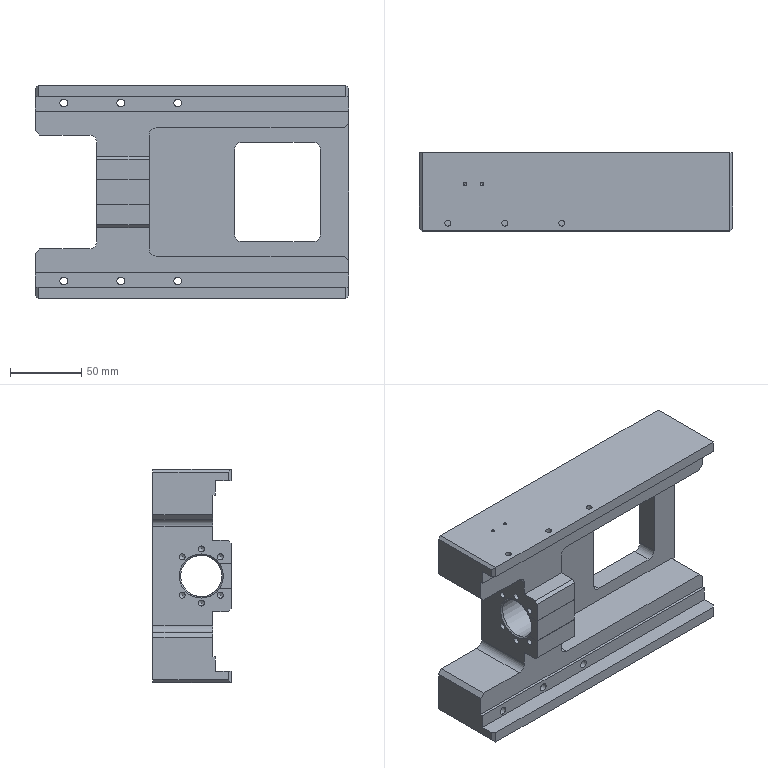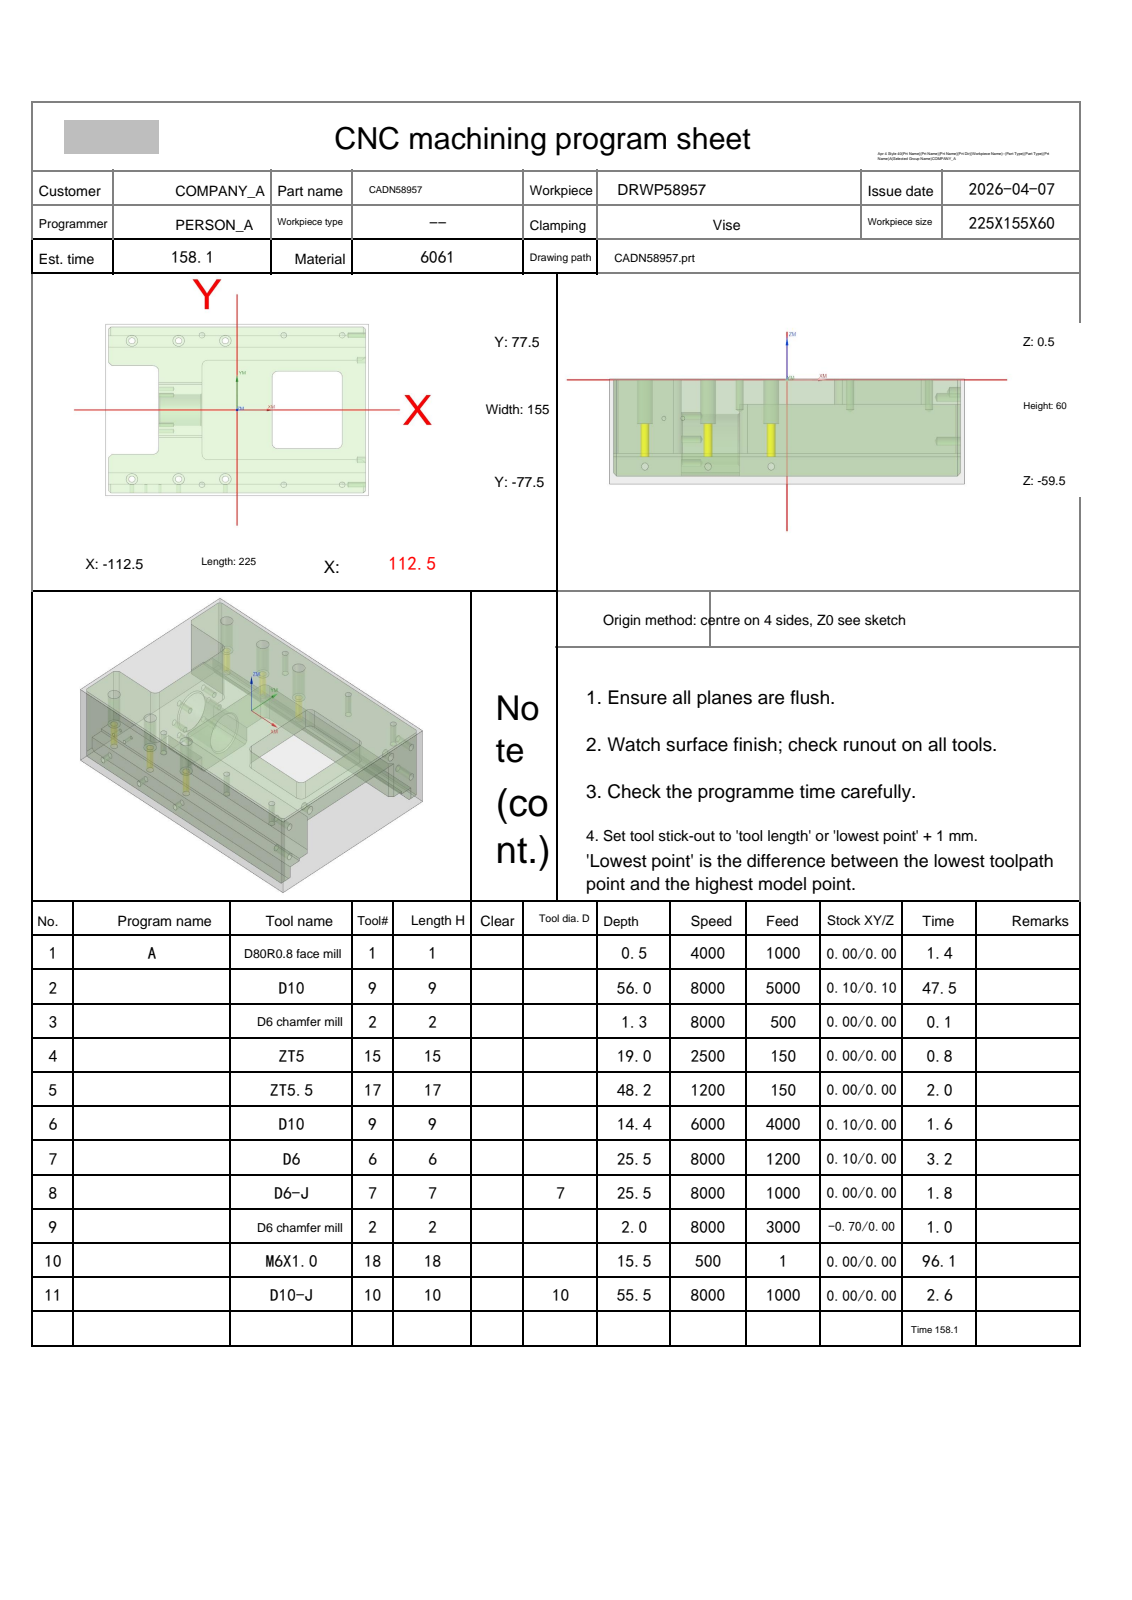NC program | NX | posted by the shop | part box 220 x 55 x 150 mm
Lines 1 to 41 of 12878:
%
O0001
(Machine time: 250.20 MIN)
(===Total Tool:9===)
(T1=D80R0.8 face mill D=80.  R=0.8  D-  H01 Z=-0.   )
(T9=D10     D=10.  R=0.   D-  H09 Z=-55.5 )
(T2=D6 chamfer mill   D=6.   R=0.   D-  H02 Z=-1.5  )
(T15=ZT5    D=5.   DR_a=118 D-  H15 Z=-18.5 )
(T17=ZT5.5  D=5.5  DR_a=118 D-  H17 Z=-47.65)
(T6=D6      D=6.   R=0.   D-  H06 Z=-25.  )
(T7=D6-J    D=6.   R=0.   D7  H07 Z=-25.  )
(T18=M6X1.0 D=5.   DR_a=180 D-  H18 Z=-15.  )
(T10=D10-J  D=10.  R=0.   D10 H10 Z=-55.  )
G80 G90 G17 G49 G40
G91 G28 Z0
M01
N1 T01 M06
(D80R0.8 face mill  D=80. R=0.8 H=01 ce=0.00 di=0.00)
G00 G90 G54 X155. Y-69. M03 S4000
G43 H01 Z20.
M08
Z2.
G01 Z0.0 F1000.
X150.
X-150.
Y-23.
X150.
Y23.
X-150.
Y69.
X150.
X155.
Z2.
G00 Z20.
G91 G28 Z0.0
M05
M09
G91 G28 Z0.0
M01